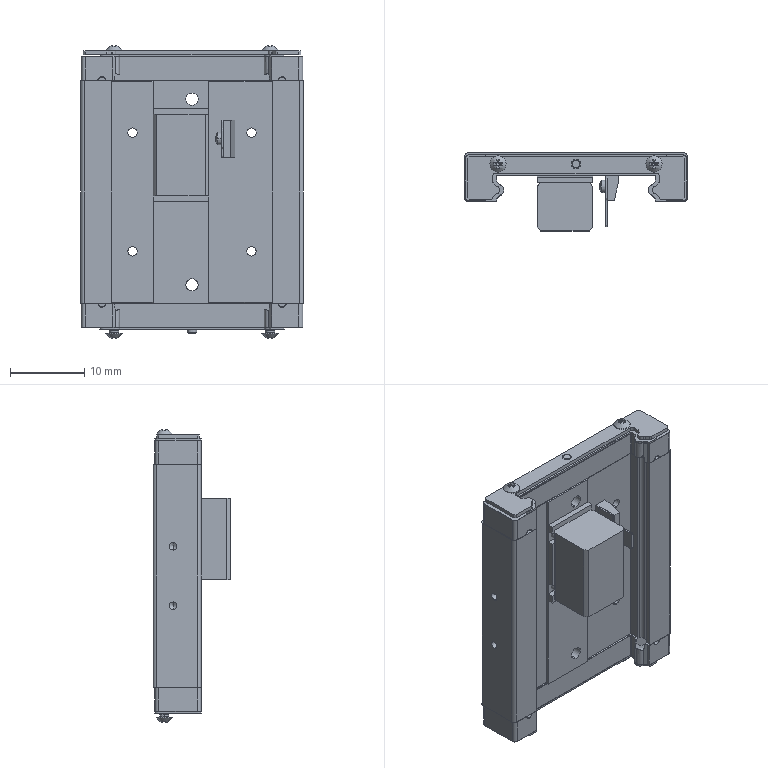Part | SolidWorks | features BaseBody 23, Scale 1 | 23 solids | 1854 faces | box 30 x 10.5 x 39.416 mm | volume 4914 mm3 | cylinder 619 | cone 467 | spline 425 | plane 343 | commonest cylinder face diameters 0.05 x248 1.25 x188 1 x37 1.65 x32 1.5 x20 0.5 x16